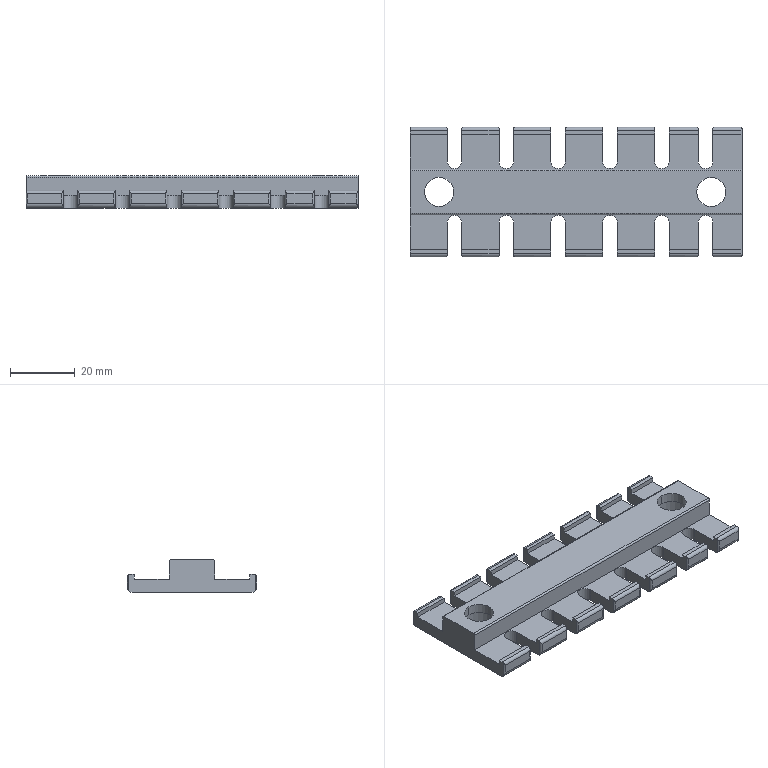Part | STEP file | ZL103 | 1 solid | 154 faces | box 102.5 x 40 x 10 mm | volume 20761 mm3 | cylinder 78 | plane 76 | commonest cylinder face diameters 1 x30 2 x14 3 x14 4.5 x12 9 x4 12 x4